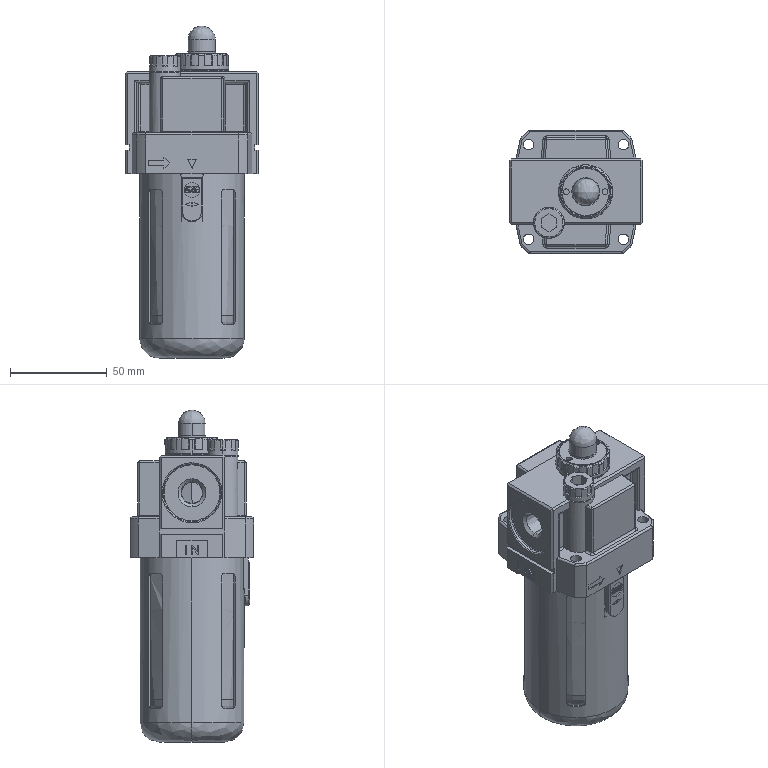Part | SolidWorks | features BaseBody 1 | 1 solid | 870 faces | box 68.8 x 64 x 171.6 mm | volume 182520 mm3 | plane 455 | cylinder 243 | cone 89 | spline 57 | torus 23 | sphere 3 | commonest cylinder face diameters 2 x63 4 x16 27 x12 14.5 x9 5.5 x8 63.8 x8